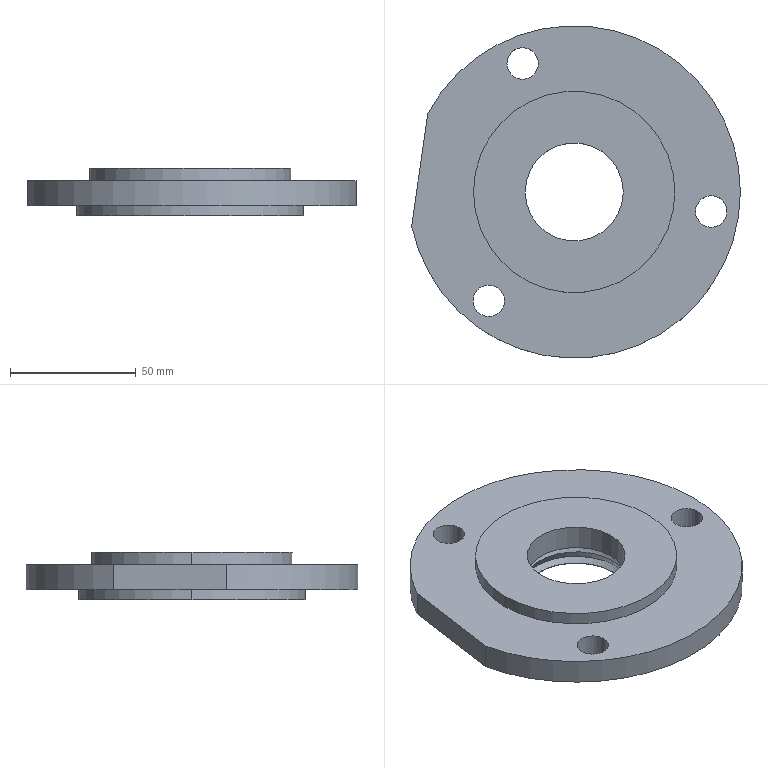Part | SolidWorks | features HoleWzd 2, Revolution 2, BaseBody 1, Extrusion 1 | 2 solids | 52 faces | box 130.573 x 132 x 19 mm | volume 150304 mm3 | cylinder 22 | torus 12 | plane 10 | cone 8 | commonest cylinder face diameters 12.5 x6 62 x4 39 x2 44.8 x2 58 x2 80 x2
STEP:
#1=CARTESIAN_POINT('',(607.231,22.744,-149.693));
#2=VERTEX_POINT('',#1);
#3=CARTESIAN_POINT('',(545.231,22.744,-149.693));
#4=VERTEX_POINT('',#3);
#5=CARTESIAN_POINT('',(576.231,22.744,-149.693));
#6=DIRECTION('',(0.,0.,-1.));
#7=DIRECTION('',(-1.,0.,0.));
#8=AXIS2_PLACEMENT_3D('',#5,#6,#7);
#9=CIRCLE('',#8,31.);
#10=EDGE_CURVE('',#2,#4,#9,.T.);
#11=ORIENTED_EDGE('',*,*,#10,.F.);
#12=CARTESIAN_POINT('',(607.231,22.744,-158.693));
#13=VERTEX_POINT('',#12);
#14=CARTESIAN_POINT('',(607.231,22.744,-158.693));
#15=DIRECTION('',(0.,0.,-1.));
#16=VECTOR('',#15,1000.);
#17=LINE('',#14,#16);
#18=EDGE_CURVE('',#2,#13,#17,.T.);
#19=ORIENTED_EDGE('',*,*,#18,.T.);
#20=CARTESIAN_POINT('',(545.231,22.744,-158.693));
#21=VERTEX_POINT('',#20);
#22=CARTESIAN_POINT('',(576.231,22.744,-158.693));
#23=DIRECTION('',(0.,0.,-1.));
#24=DIRECTION('',(-1.,0.,0.));
#25=AXIS2_PLACEMENT_3D('',#22,#23,#24);
#26=CIRCLE('',#25,31.);
#27=EDGE_CURVE('',#13,#21,#26,.T.);
#28=ORIENTED_EDGE('',*,*,#27,.T.);
#29=CARTESIAN_POINT('',(545.231,22.744,-158.693));
#30=DIRECTION('',(0.,0.,-1.));
#31=VECTOR('',#30,1000.);
#32=LINE('',#29,#31);
#33=EDGE_CURVE('',#4,#21,#32,.T.);
#34=ORIENTED_EDGE('',*,*,#33,.F.);
#35=EDGE_LOOP('',(#11,#19,#28,#34));
#36=FACE_OUTER_BOUND('',#35,.T.);
#37=CARTESIAN_POINT('',(576.231,22.744,-158.693));
#38=DIRECTION('',(0.,0.,-1.));
#39=DIRECTION('',(-1.,0.,0.));
#40=AXIS2_PLACEMENT_3D('',#37,#38,#39);
#41=CYLINDRICAL_SURFACE('',#40,31.);
#42=ADVANCED_FACE('',(#36),#41,.F.);
#43=CARTESIAN_POINT('',(595.731,22.744,-139.693));
#44=VERTEX_POINT('',#43);
#45=CARTESIAN_POINT('',(556.731,22.744,-139.693));
#46=VERTEX_POINT('',#45);
#47=CARTESIAN_POINT('',(576.231,22.744,-139.693));
#48=DIRECTION('',(0.,0.,-1.));
#49=DIRECTION('',(-1.,0.,0.));
#50=AXIS2_PLACEMENT_3D('',#47,#48,#49);
#51=CIRCLE('',#50,19.5);
#52=EDGE_CURVE('',#44,#46,#51,.T.);
#53=ORIENTED_EDGE('',*,*,#52,.F.);
#54=CARTESIAN_POINT('',(595.731,22.744,-149.693));
#55=VERTEX_POINT('',#54);
#56=CARTESIAN_POINT('',(595.731,22.744,-158.693));
#57=DIRECTION('',(0.,0.,-1.));
#58=VECTOR('',#57,1000.);
#59=LINE('',#56,#58);
#60=EDGE_CURVE('',#44,#55,#59,.T.);
#61=ORIENTED_EDGE('',*,*,#60,.T.);
#62=CARTESIAN_POINT('',(556.731,22.744,-149.693));
#63=VERTEX_POINT('',#62);
#64=CARTESIAN_POINT('',(576.231,22.744,-149.693));
#65=DIRECTION('',(0.,0.,-1.));
#66=DIRECTION('',(-1.,0.,0.));
#67=AXIS2_PLACEMENT_3D('',#64,#65,#66);
#68=CIRCLE('',#67,19.5);
#69=EDGE_CURVE('',#55,#63,#68,.T.);
#70=ORIENTED_EDGE('',*,*,#69,.T.);
#71=CARTESIAN_POINT('',(556.731,22.744,-158.693));
#72=DIRECTION('',(0.,0.,-1.));
#73=VECTOR('',#72,1000.);
#74=LINE('',#71,#73);
#75=EDGE_CURVE('',#46,#63,#74,.T.);
#76=ORIENTED_EDGE('',*,*,#75,.F.);
#77=EDGE_LOOP('',(#53,#61,#70,#76));
#78=FACE_OUTER_BOUND('',#77,.T.);
#79=CARTESIAN_POINT('',(576.231,22.744,-158.693));
#80=DIRECTION('',(0.,0.,-1.));
#81=DIRECTION('',(-1.,0.,0.));
#82=AXIS2_PLACEMENT_3D('',#79,#80,#81);
#83=CYLINDRICAL_SURFACE('',#82,19.5);
#84=ADVANCED_FACE('',(#78),#83,.F.);
#85=CARTESIAN_POINT('',(624.43,14.98,-144.693));
#86=VERTEX_POINT('',#85);
#87=CARTESIAN_POINT('',(636.93,14.98,-144.693));
#88=VERTEX_POINT('',#87);
#89=CARTESIAN_POINT('',(630.68,14.98,-144.693));
#90=DIRECTION('',(0.,0.,1.));
#91=DIRECTION('',(1.,0.,0.));
#92=AXIS2_PLACEMENT_3D('',#89,#90,#91);
#93=CIRCLE('',#92,6.25);
#94=EDGE_CURVE('',#86,#88,#93,.T.);
#95=ORIENTED_EDGE('',*,*,#94,.T.);
#96=CARTESIAN_POINT('',(636.93,14.98,-154.693));
#97=VERTEX_POINT('',#96);
#98=CARTESIAN_POINT('',(636.93,14.98,-154.693));
#99=DIRECTION('',(0.,0.,-1.));
#100=VECTOR('',#99,1000.);
#101=LINE('',#98,#100);
#102=EDGE_CURVE('',#88,#97,#101,.T.);
#103=ORIENTED_EDGE('',*,*,#102,.T.);
#104=CARTESIAN_POINT('',(624.43,14.98,-154.693));
#105=VERTEX_POINT('',#104);
#106=CARTESIAN_POINT('',(630.68,14.98,-154.693));
#107=DIRECTION('',(0.,0.,-1.));
#108=DIRECTION('',(-1.,0.,0.));
#109=AXIS2_PLACEMENT_3D('',#106,#107,#108);
#110=CIRCLE('',#109,6.25);
#111=EDGE_CURVE('',#97,#105,#110,.T.);
#112=ORIENTED_EDGE('',*,*,#111,.T.);
#113=CARTESIAN_POINT('',(624.43,14.98,-154.693));
#114=DIRECTION('',(0.,0.,-1.));
#115=VECTOR('',#114,1000.);
#116=LINE('',#113,#115);
#117=EDGE_CURVE('',#86,#105,#116,.T.);
#118=ORIENTED_EDGE('',*,*,#117,.F.);
#119=EDGE_LOOP('',(#95,#103,#112,#118));
#120=FACE_OUTER_BOUND('',#119,.T.);
#121=CARTESIAN_POINT('',(630.68,14.98,-154.693));
#122=DIRECTION('',(0.,0.,-1.));
#123=DIRECTION('',(-1.,0.,0.));
#124=AXIS2_PLACEMENT_3D('',#121,#122,#123);
#125=CYLINDRICAL_SURFACE('',#124,6.25);
#126=ADVANCED_FACE('',(#120),#125,.F.);
#127=CARTESIAN_POINT('',(536.032,-20.529,-144.693));
#128=VERTEX_POINT('',#127);
#129=CARTESIAN_POINT('',(548.532,-20.529,-144.693));
#130=VERTEX_POINT('',#129);
#131=CARTESIAN_POINT('',(542.282,-20.529,-144.693));
#132=DIRECTION('',(0.,0.,1.));
#133=DIRECTION('',(1.,0.,0.));
#134=AXIS2_PLACEMENT_3D('',#131,#132,#133);
#135=CIRCLE('',#134,6.25);
#136=EDGE_CURVE('',#128,#130,#135,.T.);
#137=ORIENTED_EDGE('',*,*,#136,.T.);
#138=CARTESIAN_POINT('',(548.532,-20.529,-154.693));
#139=VERTEX_POINT('',#138);
#140=CARTESIAN_POINT('',(548.532,-20.529,-154.693));
#141=DIRECTION('',(0.,0.,-1.));
#142=VECTOR('',#141,1000.);
#143=LINE('',#140,#142);
#144=EDGE_CURVE('',#130,#139,#143,.T.);
#145=ORIENTED_EDGE('',*,*,#144,.T.);
#146=CARTESIAN_POINT('',(536.032,-20.529,-154.693));
#147=VERTEX_POINT('',#146);
#148=CARTESIAN_POINT('',(542.282,-20.529,-154.693));
#149=DIRECTION('',(0.,0.,-1.));
#150=DIRECTION('',(-1.,0.,0.));
#151=AXIS2_PLACEMENT_3D('',#148,#149,#150);
#152=CIRCLE('',#151,6.25);
#153=EDGE_CURVE('',#139,#147,#152,.T.);
#154=ORIENTED_EDGE('',*,*,#153,.T.);
#155=CARTESIAN_POINT('',(536.032,-20.529,-154.693));
#156=DIRECTION('',(0.,0.,-1.));
#157=VECTOR('',#156,1000.);
#158=LINE('',#155,#157);
#159=EDGE_CURVE('',#128,#147,#158,.T.);
#160=ORIENTED_EDGE('',*,*,#159,.F.);
#161=EDGE_LOOP('',(#137,#145,#154,#160));
#162=FACE_OUTER_BOUND('',#161,.T.);
#163=CARTESIAN_POINT('',(542.282,-20.529,-154.693));
#164=DIRECTION('',(0.,0.,-1.));
#165=DIRECTION('',(-1.,0.,0.));
#166=AXIS2_PLACEMENT_3D('',#163,#164,#165);
#167=CYLINDRICAL_SURFACE('',#166,6.25);
#168=ADVANCED_FACE('',(#162),#167,.F.);
#169=CARTESIAN_POINT('',(549.479,73.78,-144.693));
#170=VERTEX_POINT('',#169);
#171=CARTESIAN_POINT('',(561.979,73.78,-144.693));
#172=VERTEX_POINT('',#171);
#173=CARTESIAN_POINT('',(555.729,73.78,-144.693));
#174=DIRECTION('',(0.,0.,1.));
#175=DIRECTION('',(1.,0.,0.));
#176=AXIS2_PLACEMENT_3D('',#173,#174,#175);
#177=CIRCLE('',#176,6.25);
#178=EDGE_CURVE('',#170,#172,#177,.T.);
#179=ORIENTED_EDGE('',*,*,#178,.T.);
#180=CARTESIAN_POINT('',(561.979,73.78,-154.693));
#181=VERTEX_POINT('',#180);
#182=CARTESIAN_POINT('',(561.979,73.78,-154.693));
#183=DIRECTION('',(0.,0.,-1.));
#184=VECTOR('',#183,1000.);
#185=LINE('',#182,#184);
#186=EDGE_CURVE('',#172,#181,#185,.T.);
#187=ORIENTED_EDGE('',*,*,#186,.T.);
#188=CARTESIAN_POINT('',(549.479,73.78,-154.693));
#189=VERTEX_POINT('',#188);
#190=CARTESIAN_POINT('',(555.729,73.78,-154.693));
#191=DIRECTION('',(0.,0.,-1.));
#192=DIRECTION('',(-1.,0.,0.));
#193=AXIS2_PLACEMENT_3D('',#190,#191,#192);
#194=CIRCLE('',#193,6.25);
#195=EDGE_CURVE('',#181,#189,#194,.T.);
#196=ORIENTED_EDGE('',*,*,#195,.T.);
#197=CARTESIAN_POINT('',(549.479,73.78,-154.693));
#198=DIRECTION('',(0.,0.,-1.));
#199=VECTOR('',#198,1000.);
#200=LINE('',#197,#199);
#201=EDGE_CURVE('',#170,#189,#200,.T.);
#202=ORIENTED_EDGE('',*,*,#201,.F.);
#203=EDGE_LOOP('',(#179,#187,#196,#202));
#204=FACE_OUTER_BOUND('',#203,.T.);
#205=CARTESIAN_POINT('',(555.729,73.78,-154.693));
#206=DIRECTION('',(0.,0.,-1.));
#207=DIRECTION('',(-1.,0.,0.));
#208=AXIS2_PLACEMENT_3D('',#205,#206,#207);
#209=CYLINDRICAL_SURFACE('',#208,6.25);
#210=ADVANCED_FACE('',(#204),#209,.F.);
#211=CARTESIAN_POINT('',(621.231,22.744,-158.693));
#212=VERTEX_POINT('',#211);
#213=CARTESIAN_POINT('',(531.231,22.744,-158.693));
#214=VERTEX_POINT('',#213);
#215=CARTESIAN_POINT('',(576.231,22.744,-158.693));
#216=DIRECTION('',(0.,0.,1.));
#217=DIRECTION('',(1.,0.,0.));
#218=AXIS2_PLACEMENT_3D('',#215,#216,#217);
#219=CIRCLE('',#218,45.);
#220=EDGE_CURVE('',#212,#214,#219,.T.);
#221=ORIENTED_EDGE('',*,*,#220,.T.);
#222=CARTESIAN_POINT('',(531.231,22.744,-154.693));
#223=VERTEX_POINT('',#222);
#224=CARTESIAN_POINT('',(531.231,22.744,-158.693));
#225=DIRECTION('',(0.,0.,1.));
#226=VECTOR('',#225,1000.);
#227=LINE('',#224,#226);
#228=EDGE_CURVE('',#214,#223,#227,.T.);
#229=ORIENTED_EDGE('',*,*,#228,.T.);
#230=CARTESIAN_POINT('',(621.231,22.744,-154.693));
#231=VERTEX_POINT('',#230);
#232=CARTESIAN_POINT('',(576.231,22.744,-154.693));
#233=DIRECTION('',(0.,0.,1.));
#234=DIRECTION('',(1.,0.,0.));
#235=AXIS2_PLACEMENT_3D('',#232,#233,#234);
#236=CIRCLE('',#235,45.);
#237=EDGE_CURVE('',#231,#223,#236,.T.);
#238=ORIENTED_EDGE('',*,*,#237,.F.);
#239=CARTESIAN_POINT('',(621.231,22.744,-158.693));
#240=DIRECTION('',(0.,0.,1.));
#241=VECTOR('',#240,1000.);
#242=LINE('',#239,#241);
#243=EDGE_CURVE('',#212,#231,#242,.T.);
#244=ORIENTED_EDGE('',*,*,#243,.F.);
#245=EDGE_LOOP('',(#221,#229,#238,#244));
#246=FACE_OUTER_BOUND('',#245,.T.);
#247=CARTESIAN_POINT('',(576.231,22.744,-158.693));
#248=DIRECTION('',(0.,0.,1.));
#249=DIRECTION('',(1.,0.,0.));
#250=AXIS2_PLACEMENT_3D('',#247,#248,#249);
#251=CYLINDRICAL_SURFACE('',#250,45.);
#252=ADVANCED_FACE('',(#246),#251,.T.);
#253=CARTESIAN_POINT('',(536.231,22.744,-139.693));
#254=VERTEX_POINT('',#253);
#255=CARTESIAN_POINT('',(616.231,22.744,-139.693));
#256=VERTEX_POINT('',#255);
#257=CARTESIAN_POINT('',(576.231,22.744,-139.693));
#258=DIRECTION('',(0.,0.,-1.));
#259=DIRECTION('',(-1.,0.,0.));
#260=AXIS2_PLACEMENT_3D('',#257,#258,#259);
#261=CIRCLE('',#260,40.);
#262=EDGE_CURVE('',#254,#256,#261,.T.);
#263=ORIENTED_EDGE('',*,*,#262,.T.);
#264=CARTESIAN_POINT('',(616.231,22.744,-144.693));
#265=VERTEX_POINT('',#264);
#266=CARTESIAN_POINT('',(616.231,22.744,-139.693));
#267=DIRECTION('',(0.,0.,-1.));
#268=VECTOR('',#267,1000.);
#269=LINE('',#266,#268);
#270=EDGE_CURVE('',#256,#265,#269,.T.);
#271=ORIENTED_EDGE('',*,*,#270,.T.);
#272=CARTESIAN_POINT('',(536.231,22.744,-144.693));
#273=VERTEX_POINT('',#272);
#274=CARTESIAN_POINT('',(576.231,22.744,-144.693));
#275=DIRECTION('',(0.,0.,-1.));
#276=DIRECTION('',(-1.,0.,0.));
#277=AXIS2_PLACEMENT_3D('',#274,#275,#276);
#278=CIRCLE('',#277,40.);
#279=EDGE_CURVE('',#273,#265,#278,.T.);
#280=ORIENTED_EDGE('',*,*,#279,.F.);
#281=CARTESIAN_POINT('',(536.231,22.744,-139.693));
#282=DIRECTION('',(0.,0.,-1.));
#283=VECTOR('',#282,1000.);
#284=LINE('',#281,#283);
#285=EDGE_CURVE('',#254,#273,#284,.T.);
#286=ORIENTED_EDGE('',*,*,#285,.F.);
#287=EDGE_LOOP('',(#263,#271,#280,#286));
#288=FACE_OUTER_BOUND('',#287,.T.);
#289=CARTESIAN_POINT('',(576.231,22.744,-139.693));
#290=DIRECTION('',(0.,0.,-1.));
#291=DIRECTION('',(-1.,0.,0.));
#292=AXIS2_PLACEMENT_3D('',#289,#290,#291);
#293=CYLINDRICAL_SURFACE('',#292,40.);
#294=ADVANCED_FACE('',(#288),#293,.T.);
#295=CARTESIAN_POINT('',(511.657,9.095,-154.693));
#296=VERTEX_POINT('',#295);
#297=CARTESIAN_POINT('',(642.231,22.744,-154.693));
#298=VERTEX_POINT('',#297);
#299=CARTESIAN_POINT('',(576.231,22.744,-154.693));
#300=DIRECTION('',(0.,0.,1.));
#301=DIRECTION('',(1.,0.,0.));
#302=AXIS2_PLACEMENT_3D('',#299,#300,#301);
#303=CIRCLE('',#302,66.);
#304=EDGE_CURVE('',#296,#298,#303,.T.);
#305=ORIENTED_EDGE('',*,*,#304,.T.);
#306=CARTESIAN_POINT('',(642.231,22.744,-144.693));
#307=VERTEX_POINT('',#306);
#308=CARTESIAN_POINT('',(642.231,22.744,-154.693));
#309=DIRECTION('',(0.,0.,1.));
#310=VECTOR('',#309,1000.);
#311=LINE('',#308,#310);
#312=EDGE_CURVE('',#298,#307,#311,.T.);
#313=ORIENTED_EDGE('',*,*,#312,.T.);
#314=CARTESIAN_POINT('',(511.657,9.095,-144.693));
#315=VERTEX_POINT('',#314);
#316=CARTESIAN_POINT('',(576.231,22.744,-144.693));
#317=DIRECTION('',(0.,0.,1.));
#318=DIRECTION('',(1.,0.,0.));
#319=AXIS2_PLACEMENT_3D('',#316,#317,#318);
#320=CIRCLE('',#319,66.);
#321=EDGE_CURVE('',#315,#307,#320,.T.);
#322=ORIENTED_EDGE('',*,*,#321,.F.);
#323=CARTESIAN_POINT('',(511.657,9.095,-154.693));
#324=DIRECTION('',(0.,0.,1.));
#325=VECTOR('',#324,1000.);
#326=LINE('',#323,#325);
#327=EDGE_CURVE('',#296,#315,#326,.T.);
#328=ORIENTED_EDGE('',*,*,#327,.F.);
#329=EDGE_LOOP('',(#305,#313,#322,#328));
#330=FACE_OUTER_BOUND('',#329,.T.);
#331=CARTESIAN_POINT('',(576.231,22.744,-154.693));
#332=DIRECTION('',(0.,0.,1.));
#333=DIRECTION('',(1.,0.,0.));
#334=AXIS2_PLACEMENT_3D('',#331,#332,#333);
#335=CYLINDRICAL_SURFACE('',#334,66.);
#336=ADVANCED_FACE('',(#330),#335,.T.);
#337=ORIENTED_EDGE('',*,*,#312,.F.);
#338=CARTESIAN_POINT('',(518.045,53.897,-154.693));
#339=VERTEX_POINT('',#338);
#340=CARTESIAN_POINT('',(576.231,22.744,-154.693));
#341=DIRECTION('',(0.,0.,1.));
#342=DIRECTION('',(1.,0.,0.));
#343=AXIS2_PLACEMENT_3D('',#340,#341,#342);
#344=CIRCLE('',#343,66.);
#345=EDGE_CURVE('',#298,#339,#344,.T.);
#346=ORIENTED_EDGE('',*,*,#345,.T.);
#347=CARTESIAN_POINT('',(518.045,53.897,-144.693));
#348=VERTEX_POINT('',#347);
#349=CARTESIAN_POINT('',(518.045,53.897,-154.693));
#350=DIRECTION('',(0.,0.,1.));
#351=VECTOR('',#350,1000.);
#352=LINE('',#349,#351);
#353=EDGE_CURVE('',#339,#348,#352,.T.);
#354=ORIENTED_EDGE('',*,*,#353,.T.);
#355=CARTESIAN_POINT('',(576.231,22.744,-144.693));
#356=DIRECTION('',(0.,0.,1.));
#357=DIRECTION('',(1.,0.,0.));
#358=AXIS2_PLACEMENT_3D('',#355,#356,#357);
#359=CIRCLE('',#358,66.);
#360=EDGE_CURVE('',#307,#348,#359,.T.);
#361=ORIENTED_EDGE('',*,*,#360,.F.);
#362=EDGE_LOOP('',(#337,#346,#354,#361));
#363=FACE_OUTER_BOUND('',#362,.T.);
#364=CARTESIAN_POINT('',(576.231,22.744,-154.693));
#365=DIRECTION('',(0.,0.,1.));
#366=DIRECTION('',(1.,0.,0.));
#367=AXIS2_PLACEMENT_3D('',#364,#365,#366);
#368=CYLINDRICAL_SURFACE('',#367,66.);
#369=ADVANCED_FACE('',(#363),#368,.T.);
#370=CARTESIAN_POINT('',(518.045,53.897,-144.693));
#371=DIRECTION('',(-0.1412,-0.99,0.));
#372=VECTOR('',#371,1000.);
#373=LINE('',#370,#372);
#374=EDGE_CURVE('',#348,#315,#373,.T.);
#375=ORIENTED_EDGE('',*,*,#374,.F.);
#376=ORIENTED_EDGE('',*,*,#353,.F.);
#377=CARTESIAN_POINT('',(518.045,53.897,-154.693));
#378=DIRECTION('',(-0.1412,-0.99,0.));
#379=VECTOR('',#378,1000.);
#380=LINE('',#377,#379);
#381=EDGE_CURVE('',#339,#296,#380,.T.);
#382=ORIENTED_EDGE('',*,*,#381,.T.);
#383=ORIENTED_EDGE('',*,*,#327,.T.);
#384=EDGE_LOOP('',(#375,#376,#382,#383));
#385=FACE_OUTER_BOUND('',#384,.T.);
#386=CARTESIAN_POINT('',(518.045,53.897,-154.693));
#387=DIRECTION('',(-0.99,0.1412,0.));
#388=DIRECTION('',(-0.1412,-0.99,0.));
#389=AXIS2_PLACEMENT_3D('',#386,#387,#388);
#390=PLANE('',#389);
#391=ADVANCED_FACE('',(#385),#390,.T.);
#392=CARTESIAN_POINT('',(630.68,14.98,-154.693));
#393=DIRECTION('',(0.,0.,-1.));
#394=DIRECTION('',(-1.,0.,0.));
#395=AXIS2_PLACEMENT_3D('',#392,#393,#394);
#396=CIRCLE('',#395,6.25);
#397=EDGE_CURVE('',#105,#97,#396,.T.);
#398=ORIENTED_EDGE('',*,*,#397,.F.);
#399=ORIENTED_EDGE('',*,*,#111,.F.);
#400=EDGE_LOOP('',(#398,#399));
#401=FACE_BOUND('',#400,.T.);
#402=CARTESIAN_POINT('',(542.282,-20.529,-154.693));
#403=DIRECTION('',(0.,0.,-1.));
#404=DIRECTION('',(-1.,0.,0.));
#405=AXIS2_PLACEMENT_3D('',#402,#403,#404);
#406=CIRCLE('',#405,6.25);
#407=EDGE_CURVE('',#147,#139,#406,.T.);
#408=ORIENTED_EDGE('',*,*,#407,.F.);
#409=ORIENTED_EDGE('',*,*,#153,.F.);
#410=EDGE_LOOP('',(#408,#409));
#411=FACE_BOUND('',#410,.T.);
#412=CARTESIAN_POINT('',(555.729,73.78,-154.693));
#413=DIRECTION('',(0.,0.,-1.));
#414=DIRECTION('',(-1.,0.,0.));
#415=AXIS2_PLACEMENT_3D('',#412,#413,#414);
#416=CIRCLE('',#415,6.25);
#417=EDGE_CURVE('',#189,#181,#416,.T.);
#418=ORIENTED_EDGE('',*,*,#417,.F.);
#419=ORIENTED_EDGE('',*,*,#195,.F.);
#420=EDGE_LOOP('',(#418,#419));
#421=FACE_BOUND('',#420,.T.);
#422=ORIENTED_EDGE('',*,*,#237,.T.);
#423=CARTESIAN_POINT('',(576.231,22.744,-154.693));
#424=DIRECTION('',(0.,0.,1.));
#425=DIRECTION('',(1.,0.,0.));
#426=AXIS2_PLACEMENT_3D('',#423,#424,#425);
#427=CIRCLE('',#426,45.);
#428=EDGE_CURVE('',#223,#231,#427,.T.);
#429=ORIENTED_EDGE('',*,*,#428,.T.);
#430=EDGE_LOOP('',(#422,#429));
#431=FACE_BOUND('',#430,.T.);
#432=ORIENTED_EDGE('',*,*,#304,.F.);
#433=ORIENTED_EDGE('',*,*,#381,.F.);
#434=ORIENTED_EDGE('',*,*,#345,.F.);
#435=EDGE_LOOP('',(#432,#433,#434));
#436=FACE_OUTER_BOUND('',#435,.T.);
#437=CARTESIAN_POINT('',(576.231,22.744,-154.693));
#438=DIRECTION('',(0.,0.,1.));
#439=DIRECTION('',(1.,0.,0.));
#440=AXIS2_PLACEMENT_3D('',#437,#438,#439);
#441=PLANE('',#440);
#442=ADVANCED_FACE('',(#401,#411,#421,#431,#436),#441,.F.);
#443=ORIENTED_EDGE('',*,*,#94,.F.);
#444=CARTESIAN_POINT('',(630.68,14.98,-144.693));
#445=DIRECTION('',(0.,0.,1.));
#446=DIRECTION('',(1.,0.,0.));
#447=AXIS2_PLACEMENT_3D('',#444,#445,#446);
#448=CIRCLE('',#447,6.25);
#449=EDGE_CURVE('',#88,#86,#448,.T.);
#450=ORIENTED_EDGE('',*,*,#449,.F.);
#451=EDGE_LOOP('',(#443,#450));
#452=FACE_BOUND('',#451,.T.);
#453=ORIENTED_EDGE('',*,*,#136,.F.);
#454=CARTESIAN_POINT('',(542.282,-20.529,-144.693));
#455=DIRECTION('',(0.,0.,1.));
#456=DIRECTION('',(1.,0.,0.));
#457=AXIS2_PLACEMENT_3D('',#454,#455,#456);
#458=CIRCLE('',#457,6.25);
#459=EDGE_CURVE('',#130,#128,#458,.T.);
#460=ORIENTED_EDGE('',*,*,#459,.F.);
#461=EDGE_LOOP('',(#453,#460));
#462=FACE_BOUND('',#461,.T.);
#463=ORIENTED_EDGE('',*,*,#178,.F.);
#464=CARTESIAN_POINT('',(555.729,73.78,-144.693));
#465=DIRECTION('',(0.,0.,1.));
#466=DIRECTION('',(1.,0.,0.));
#467=AXIS2_PLACEMENT_3D('',#464,#465,#466);
#468=CIRCLE('',#467,6.25);
#469=EDGE_CURVE('',#172,#170,#468,.T.);
#470=ORIENTED_EDGE('',*,*,#469,.F.);
#471=EDGE_LOOP('',(#463,#470));
#472=FACE_BOUND('',#471,.T.);
#473=ORIENTED_EDGE('',*,*,#279,.T.);
#474=CARTESIAN_POINT('',(576.231,22.744,-144.693));
#475=DIRECTION('',(0.,0.,-1.));
#476=DIRECTION('',(-1.,0.,0.));
#477=AXIS2_PLACEMENT_3D('',#474,#475,#476);
#478=CIRCLE('',#477,40.);
#479=EDGE_CURVE('',#265,#273,#478,.T.);
#480=ORIENTED_EDGE('',*,*,#479,.T.);
#481=EDGE_LOOP('',(#473,#480));
#482=FACE_BOUND('',#481,.T.);
#483=ORIENTED_EDGE('',*,*,#321,.T.);
#484=ORIENTED_EDGE('',*,*,#360,.T.);
#485=ORIENTED_EDGE('',*,*,#374,.T.);
#486=EDGE_LOOP('',(#483,#484,#485));
#487=FACE_OUTER_BOUND('',#486,.T.);
#488=CARTESIAN_POINT('',(576.231,22.744,-144.693));
#489=DIRECTION('',(0.,0.,1.));
#490=DIRECTION('',(1.,0.,0.));
#491=AXIS2_PLACEMENT_3D('',#488,#489,#490);
#492=PLANE('',#491);
#493=ADVANCED_FACE('',(#452,#462,#472,#482,#487),#492,.T.);
#494=ORIENTED_EDGE('',*,*,#270,.F.);
#495=CARTESIAN_POINT('',(576.231,22.744,-139.693));
#496=DIRECTION('',(0.,0.,-1.));
#497=DIRECTION('',(-1.,0.,0.));
#498=AXIS2_PLACEMENT_3D('',#495,#496,#497);
#499=CIRCLE('',#498,40.);
#500=EDGE_CURVE('',#256,#254,#499,.T.);
#501=ORIENTED_EDGE('',*,*,#500,.T.);
#502=ORIENTED_EDGE('',*,*,#285,.T.);
#503=ORIENTED_EDGE('',*,*,#479,.F.);
#504=EDGE_LOOP('',(#494,#501,#502,#503));
#505=FACE_OUTER_BOUND('',#504,.T.);
#506=CARTESIAN_POINT('',(576.231,22.744,-139.693));
#507=DIRECTION('',(0.,0.,-1.));
#508=DIRECTION('',(-1.,0.,0.));
#509=AXIS2_PLACEMENT_3D('',#506,#507,#508);
#510=CYLINDRICAL_SURFACE('',#509,40.);
#511=ADVANCED_FACE('',(#505),#510,.T.);
#512=CARTESIAN_POINT('',(576.231,22.744,-139.693));
#513=DIRECTION('',(0.,0.,-1.));
#514=DIRECTION('',(-1.,0.,0.));
#515=AXIS2_PLACEMENT_3D('',#512,#513,#514);
#516=CIRCLE('',#515,19.5);
#517=EDGE_CURVE('',#46,#44,#516,.T.);
#518=ORIENTED_EDGE('',*,*,#517,.T.);
#519=ORIENTED_EDGE('',*,*,#52,.T.);
#520=EDGE_LOOP('',(#518,#519));
#521=FACE_BOUND('',#520,.T.);
#522=ORIENTED_EDGE('',*,*,#262,.F.);
#523=ORIENTED_EDGE('',*,*,#500,.F.);
#524=EDGE_LOOP('',(#522,#523));
#525=FACE_OUTER_BOUND('',#524,.T.);
#526=CARTESIAN_POINT('',(616.231,22.744,-139.693));
#527=DIRECTION('',(0.,0.,1.));
#528=DIRECTION('',(1.,0.,0.));
#529=AXIS2_PLACEMENT_3D('',#526,#527,#528);
#530=PLANE('',#529);
#531=ADVANCED_FACE('',(#521,#525),#530,.T.);
#532=ORIENTED_EDGE('',*,*,#228,.F.);
#533=CARTESIAN_POINT('',(576.231,22.744,-158.693));
#534=DIRECTION('',(0.,0.,1.));
#535=DIRECTION('',(1.,0.,0.));
#536=AXIS2_PLACEMENT_3D('',#533,#534,#535);
#537=CIRCLE('',#536,45.);
#538=EDGE_CURVE('',#214,#212,#537,.T.);
#539=ORIENTED_EDGE('',*,*,#538,.T.);
#540=ORIENTED_EDGE('',*,*,#243,.T.);
#541=ORIENTED_EDGE('',*,*,#428,.F.);
#542=EDGE_LOOP('',(#532,#539,#540,#541));
#543=FACE_OUTER_BOUND('',#542,.T.);
#544=CARTESIAN_POINT('',(576.231,22.744,-158.693));
#545=DIRECTION('',(0.,0.,1.));
#546=DIRECTION('',(1.,0.,0.));
#547=AXIS2_PLACEMENT_3D('',#544,#545,#546);
#548=CYLINDRICAL_SURFACE('',#547,45.);
#549=ADVANCED_FACE('',(#543),#548,.T.);
#550=CARTESIAN_POINT('',(576.231,22.744,-158.693));
#551=DIRECTION('',(0.,0.,-1.));
#552=DIRECTION('',(-1.,0.,0.));
#553=AXIS2_PLACEMENT_3D('',#550,#551,#552);
#554=CIRCLE('',#553,31.);
#555=EDGE_CURVE('',#21,#13,#554,.T.);
#556=ORIENTED_EDGE('',*,*,#555,.F.);
#557=ORIENTED_EDGE('',*,*,#27,.F.);
#558=EDGE_LOOP('',(#556,#557));
#559=FACE_BOUND('',#558,.T.);
#560=ORIENTED_EDGE('',*,*,#220,.F.);
#561=ORIENTED_EDGE('',*,*,#538,.F.);
#562=EDGE_LOOP('',(#560,#561));
#563=FACE_OUTER_BOUND('',#562,.T.);
#564=CARTESIAN_POINT('',(621.231,22.744,-158.693));
#565=DIRECTION('',(0.,0.,-1.));
#566=DIRECTION('',(-1.,0.,0.));
#567=AXIS2_PLACEMENT_3D('',#564,#565,#566);
#568=PLANE('',#567);
#569=ADVANCED_FACE('',(#559,#563),#568,.T.);
#570=ORIENTED_EDGE('',*,*,#186,.F.);
#571=ORIENTED_EDGE('',*,*,#469,.T.);
#572=ORIENTED_EDGE('',*,*,#201,.T.);
#573=ORIENTED_EDGE('',*,*,#417,.T.);
#574=EDGE_LOOP('',(#570,#571,#572,#573));
#575=FACE_OUTER_BOUND('',#574,.T.);
#576=CARTESIAN_POINT('',(555.729,73.78,-154.693));
#577=DIRECTION('',(0.,0.,-1.));
#578=DIRECTION('',(-1.,0.,0.));
#579=AXIS2_PLACEMENT_3D('',#576,#577,#578);
#580=CYLINDRICAL_SURFACE('',#579,6.25);
#581=ADVANCED_FACE('',(#575),#580,.F.);
#582=ORIENTED_EDGE('',*,*,#144,.F.);
#583=ORIENTED_EDGE('',*,*,#459,.T.);
#584=ORIENTED_EDGE('',*,*,#159,.T.);
#585=ORIENTED_EDGE('',*,*,#407,.T.);
#586=EDGE_LOOP('',(#582,#583,#584,#585));
#587=FACE_OUTER_BOUND('',#586,.T.);
#588=CARTESIAN_POINT('',(542.282,-20.529,-154.693));
#589=DIRECTION('',(0.,0.,-1.));
#590=DIRECTION('',(-1.,0.,0.));
#591=AXIS2_PLACEMENT_3D('',#588,#589,#590);
#592=CYLINDRICAL_SURFACE('',#591,6.25);
#593=ADVANCED_FACE('',(#587),#592,.F.);
#594=ORIENTED_EDGE('',*,*,#102,.F.);
#595=ORIENTED_EDGE('',*,*,#449,.T.);
#596=ORIENTED_EDGE('',*,*,#117,.T.);
#597=ORIENTED_EDGE('',*,*,#397,.T.);
#598=EDGE_LOOP('',(#594,#595,#596,#597));
#599=FACE_OUTER_BOUND('',#598,.T.);
#600=CARTESIAN_POINT('',(630.68,14.98,-154.693));
#601=DIRECTION('',(0.,0.,-1.));
#602=DIRECTION('',(-1.,0.,0.));
#603=AXIS2_PLACEMENT_3D('',#600,#601,#602);
#604=CYLINDRICAL_SURFACE('',#603,6.25);
#605=ADVANCED_FACE('',(#599),#604,.F.);
#606=ORIENTED_EDGE('',*,*,#60,.F.);
#607=ORIENTED_EDGE('',*,*,#517,.F.);
#608=ORIENTED_EDGE('',*,*,#75,.T.);
#609=CARTESIAN_POINT('',(576.231,22.744,-149.693));
#610=DIRECTION('',(0.,0.,-1.));
#611=DIRECTION('',(-1.,0.,0.));
#612=AXIS2_PLACEMENT_3D('',#609,#610,#611);
#613=CIRCLE('',#612,19.5);
#614=EDGE_CURVE('',#63,#55,#613,.T.);
#615=ORIENTED_EDGE('',*,*,#614,.T.);
#616=EDGE_LOOP('',(#606,#607,#608,#615));
#617=FACE_OUTER_BOUND('',#616,.T.);
#618=CARTESIAN_POINT('',(576.231,22.744,-158.693));
#619=DIRECTION('',(0.,0.,-1.));
#620=DIRECTION('',(-1.,0.,0.));
#621=AXIS2_PLACEMENT_3D('',#618,#619,#620);
#622=CYLINDRICAL_SURFACE('',#621,19.5);
#623=ADVANCED_FACE('',(#617),#622,.F.);
#624=ORIENTED_EDGE('',*,*,#614,.F.);
#625=ORIENTED_EDGE('',*,*,#69,.F.);
#626=EDGE_LOOP('',(#624,#625));
#627=FACE_BOUND('',#626,.T.);
#628=CARTESIAN_POINT('',(576.231,22.744,-149.693));
#629=DIRECTION('',(0.,0.,-1.));
#630=DIRECTION('',(-1.,0.,0.));
#631=AXIS2_PLACEMENT_3D('',#628,#629,#630);
#632=CIRCLE('',#631,31.);
#633=EDGE_CURVE('',#4,#2,#632,.T.);
#634=ORIENTED_EDGE('',*,*,#633,.T.);
#635=ORIENTED_EDGE('',*,*,#10,.T.);
#636=EDGE_LOOP('',(#634,#635));
#637=FACE_OUTER_BOUND('',#636,.T.);
#638=CARTESIAN_POINT('',(595.731,22.744,-149.693));
#639=DIRECTION('',(0.,0.,1.));
#640=DIRECTION('',(1.,0.,0.));
#641=AXIS2_PLACEMENT_3D('',#638,#639,#640);
#642=PLANE('',#641);
#643=ADVANCED_FACE('',(#627,#637),#642,.F.);
#644=ORIENTED_EDGE('',*,*,#18,.F.);
#645=ORIENTED_EDGE('',*,*,#633,.F.);
#646=ORIENTED_EDGE('',*,*,#33,.T.);
#647=ORIENTED_EDGE('',*,*,#555,.T.);
#648=EDGE_LOOP('',(#644,#645,#646,#647));
#649=FACE_OUTER_BOUND('',#648,.T.);
#650=CARTESIAN_POINT('',(576.231,22.744,-158.693));
#651=DIRECTION('',(0.,0.,-1.));
#652=DIRECTION('',(-1.,0.,0.));
#653=AXIS2_PLACEMENT_3D('',#650,#651,#652);
#654=CYLINDRICAL_SURFACE('',#653,31.);
#655=ADVANCED_FACE('',(#649),#654,.F.);
#656=CLOSED_SHELL('',(#42,#84,#126,#168,#210,#252,#294,#336,#369,#391,#442,#493,#511,#531,#549,#569,#581,#593,#605,#623,#643,#655));
#657=MANIFOLD_SOLID_BREP('',#656);
#658=CARTESIAN_POINT('',(591.139,9.412,-157.604));
#659=VERTEX_POINT('',#658);
#660=CARTESIAN_POINT('',(591.16,9.394,-157.539));
#661=VERTEX_POINT('',#660);
#662=CARTESIAN_POINT('',(591.206,9.353,-157.604));
#663=DIRECTION('',(0.6666,0.7454,0.));
#664=DIRECTION('',(-0.7454,0.6666,0.));
#665=AXIS2_PLACEMENT_3D('',#662,#663,#664);
#666=CIRCLE('',#665,0.08889);
#667=EDGE_CURVE('',#659,#661,#666,.T.);
#668=ORIENTED_EDGE('',*,*,#667,.F.);
#669=CARTESIAN_POINT('',(561.322,36.076,-157.604));
#670=VERTEX_POINT('',#669);
#671=CARTESIAN_POINT('',(576.231,22.744,-157.604));
#672=DIRECTION('',(0.,0.,-1.));
#673=DIRECTION('',(-1.,0.,0.));
#674=AXIS2_PLACEMENT_3D('',#671,#672,#673);
#675=CIRCLE('',#674,20.);
#676=EDGE_CURVE('',#659,#670,#675,.T.);
#677=ORIENTED_EDGE('',*,*,#676,.T.);
#678=CARTESIAN_POINT('',(561.301,36.094,-157.539));
#679=VERTEX_POINT('',#678);
#680=CARTESIAN_POINT('',(561.256,36.135,-157.604));
#681=DIRECTION('',(-0.6666,-0.7454,0.));
#682=DIRECTION('',(0.7454,-0.6666,0.));
#683=AXIS2_PLACEMENT_3D('',#680,#681,#682);
#684=CIRCLE('',#683,0.08889);
#685=EDGE_CURVE('',#670,#679,#684,.T.);
#686=ORIENTED_EDGE('',*,*,#685,.T.);
#687=CARTESIAN_POINT('',(576.231,22.744,-157.539));
#688=DIRECTION('',(0.,0.,-1.));
#689=DIRECTION('',(-0.7454,0.6666,0.));
#690=AXIS2_PLACEMENT_3D('',#687,#688,#689);
#691=CIRCLE('',#690,20.028);
#692=EDGE_CURVE('',#661,#679,#691,.T.);
#693=ORIENTED_EDGE('',*,*,#692,.F.);
#694=EDGE_LOOP('',(#668,#677,#686,#693));
#695=FACE_OUTER_BOUND('',#694,.T.);
#696=CARTESIAN_POINT('',(576.231,22.744,-157.604));
#697=DIRECTION('',(0.,0.,-1.));
#698=DIRECTION('',(-0.7454,0.6666,0.));
#699=AXIS2_PLACEMENT_3D('',#696,#697,#698);
#700=TOROIDAL_SURFACE('',#699,20.089,0.08889);
#701=ADVANCED_FACE('',(#695),#700,.T.);
#702=ORIENTED_EDGE('',*,*,#685,.F.);
#703=CARTESIAN_POINT('',(576.231,22.744,-157.604));
#704=DIRECTION('',(0.,0.,-1.));
#705=DIRECTION('',(-1.,0.,0.));
#706=AXIS2_PLACEMENT_3D('',#703,#704,#705);
#707=CIRCLE('',#706,20.);
#708=EDGE_CURVE('',#670,#659,#707,.T.);
#709=ORIENTED_EDGE('',*,*,#708,.T.);
#710=ORIENTED_EDGE('',*,*,#667,.T.);
#711=CARTESIAN_POINT('',(576.231,22.744,-157.539));
#712=DIRECTION('',(0.,0.,-1.));
#713=DIRECTION('',(-0.7454,0.6666,0.));
#714=AXIS2_PLACEMENT_3D('',#711,#712,#713);
#715=CIRCLE('',#714,20.028);
#716=EDGE_CURVE('',#679,#661,#715,.T.);
#717=ORIENTED_EDGE('',*,*,#716,.F.);
#718=EDGE_LOOP('',(#702,#709,#710,#717));
#719=FACE_OUTER_BOUND('',#718,.T.);
#720=CARTESIAN_POINT('',(576.231,22.744,-157.604));
#721=DIRECTION('',(0.,0.,-1.));
#722=DIRECTION('',(-0.7454,0.6666,0.));
#723=AXIS2_PLACEMENT_3D('',#720,#721,#722);
#724=TOROIDAL_SURFACE('',#723,20.089,0.08889);
#725=ADVANCED_FACE('',(#719),#724,.T.);
#726=CARTESIAN_POINT('',(591.139,9.412,-152.093));
#727=VERTEX_POINT('',#726);
#728=CARTESIAN_POINT('',(561.322,36.076,-152.093));
#729=VERTEX_POINT('',#728);
#730=CARTESIAN_POINT('',(576.231,22.744,-152.093));
#731=DIRECTION('',(0.,0.,-1.));
#732=DIRECTION('',(-0.7454,0.6666,0.));
#733=AXIS2_PLACEMENT_3D('',#730,#731,#732);
#734=CIRCLE('',#733,20.);
#735=EDGE_CURVE('',#727,#729,#734,.T.);
#736=ORIENTED_EDGE('',*,*,#735,.T.);
#737=CARTESIAN_POINT('',(560.605,36.716,-150.493));
#738=VERTEX_POINT('',#737);
#739=CARTESIAN_POINT('',(561.322,36.076,-152.093));
#740=DIRECTION('',(-0.3839,0.3433,0.8572));
#741=VECTOR('',#740,1000.);
#742=LINE('',#739,#741);
#743=EDGE_CURVE('',#729,#738,#742,.T.);
#744=ORIENTED_EDGE('',*,*,#743,.T.);
#745=CARTESIAN_POINT('',(591.856,8.771,-150.493));
#746=VERTEX_POINT('',#745);
#747=CARTESIAN_POINT('',(576.231,22.744,-150.493));
#748=DIRECTION('',(0.,0.,-1.));
#749=DIRECTION('',(-0.7454,0.6666,0.));
#750=AXIS2_PLACEMENT_3D('',#747,#748,#749);
#751=CIRCLE('',#750,20.961);
#752=EDGE_CURVE('',#746,#738,#751,.T.);
#753=ORIENTED_EDGE('',*,*,#752,.F.);
#754=CARTESIAN_POINT('',(591.139,9.412,-152.093));
#755=DIRECTION('',(0.3839,-0.3433,0.8572));
#756=VECTOR('',#755,1000.);
#757=LINE('',#754,#756);
#758=EDGE_CURVE('',#727,#746,#757,.T.);
#759=ORIENTED_EDGE('',*,*,#758,.F.);
#760=EDGE_LOOP('',(#736,#744,#753,#759));
#761=FACE_OUTER_BOUND('',#760,.T.);
#762=CARTESIAN_POINT('',(576.231,22.744,-152.093));
#763=DIRECTION('',(0.,0.,1.));
#764=DIRECTION('',(0.7454,-0.6666,0.));
#765=AXIS2_PLACEMENT_3D('',#762,#763,#764);
#766=CONICAL_SURFACE('',#765,20.,0.5411);
#767=ADVANCED_FACE('',(#761),#766,.F.);
#768=ORIENTED_EDGE('',*,*,#735,.F.);
#769=CARTESIAN_POINT('',(592.63,8.079,-155.693));
#770=VERTEX_POINT('',#769);
#771=CARTESIAN_POINT('',(592.63,8.079,-155.693));
#772=DIRECTION('',(0.362,-0.3237,-0.8742));
#773=VECTOR('',#772,1000.);
#774=LINE('',#771,#773);
#775=EDGE_CURVE('',#727,#770,#774,.T.);
#776=ORIENTED_EDGE('',*,*,#775,.T.);
#777=CARTESIAN_POINT('',(559.831,37.409,-155.693));
#778=VERTEX_POINT('',#777);
#779=CARTESIAN_POINT('',(576.231,22.744,-155.693));
#780=DIRECTION('',(0.,0.,-1.));
#781=DIRECTION('',(-0.7454,0.6666,0.));
#782=AXIS2_PLACEMENT_3D('',#779,#780,#781);
#783=CIRCLE('',#782,22.);
#784=EDGE_CURVE('',#770,#778,#783,.T.);
#785=ORIENTED_EDGE('',*,*,#784,.T.);
#786=CARTESIAN_POINT('',(559.831,37.409,-155.693));
#787=DIRECTION('',(-0.362,0.3237,-0.8742));
#788=VECTOR('',#787,1000.);
#789=LINE('',#786,#788);
#790=EDGE_CURVE('',#729,#778,#789,.T.);
#791=ORIENTED_EDGE('',*,*,#790,.F.);
#792=EDGE_LOOP('',(#768,#776,#785,#791));
#793=FACE_OUTER_BOUND('',#792,.T.);
#794=CARTESIAN_POINT('',(576.231,22.744,-155.693));
#795=DIRECTION('',(0.,0.,-1.));
#796=DIRECTION('',(-0.7454,0.6666,0.));
#797=AXIS2_PLACEMENT_3D('',#794,#795,#796);
#798=CONICAL_SURFACE('',#797,22.,0.5071);
#799=ADVANCED_FACE('',(#793),#798,.F.);
#800=ORIENTED_EDGE('',*,*,#692,.T.);
#801=CARTESIAN_POINT('',(561.301,36.094,-157.539));
#802=DIRECTION('',(-0.5441,0.4866,0.6835));
#803=VECTOR('',#802,1000.);
#804=LINE('',#801,#803);
#805=EDGE_CURVE('',#679,#778,#804,.T.);
#806=ORIENTED_EDGE('',*,*,#805,.T.);
#807=ORIENTED_EDGE('',*,*,#784,.F.);
#808=CARTESIAN_POINT('',(591.16,9.394,-157.539));
#809=DIRECTION('',(0.5441,-0.4866,0.6835));
#810=VECTOR('',#809,1000.);
#811=LINE('',#808,#810);
#812=EDGE_CURVE('',#661,#770,#811,.T.);
#813=ORIENTED_EDGE('',*,*,#812,.F.);
#814=EDGE_LOOP('',(#800,#806,#807,#813));
#815=FACE_OUTER_BOUND('',#814,.T.);
#816=CARTESIAN_POINT('',(576.231,22.744,-157.539));
#817=DIRECTION('',(0.,0.,1.));
#818=DIRECTION('',(0.7454,-0.6666,0.));
#819=AXIS2_PLACEMENT_3D('',#816,#817,#818);
#820=CONICAL_SURFACE('',#819,20.028,0.8183);
#821=ADVANCED_FACE('',(#815),#820,.F.);
#822=ORIENTED_EDGE('',*,*,#708,.F.);
#823=CARTESIAN_POINT('',(561.256,36.135,-157.693));
#824=VERTEX_POINT('',#823);
#825=CARTESIAN_POINT('',(561.256,36.135,-157.604));
#826=DIRECTION('',(-0.6666,-0.7454,0.));
#827=DIRECTION('',(0.7454,-0.6666,0.));
#828=AXIS2_PLACEMENT_3D('',#825,#826,#827);
#829=CIRCLE('',#828,0.08889);
#830=EDGE_CURVE('',#824,#670,#829,.T.);
#831=ORIENTED_EDGE('',*,*,#830,.F.);
#832=CARTESIAN_POINT('',(591.206,9.353,-157.693));
#833=VERTEX_POINT('',#832);
#834=CARTESIAN_POINT('',(576.231,22.744,-157.693));
#835=DIRECTION('',(0.,0.,-1.));
#836=DIRECTION('',(-0.7454,0.6666,0.));
#837=AXIS2_PLACEMENT_3D('',#834,#835,#836);
#838=CIRCLE('',#837,20.089);
#839=EDGE_CURVE('',#824,#833,#838,.T.);
#840=ORIENTED_EDGE('',*,*,#839,.T.);
#841=CARTESIAN_POINT('',(591.206,9.353,-157.604));
#842=DIRECTION('',(0.6666,0.7454,0.));
#843=DIRECTION('',(-0.7454,0.6666,0.));
#844=AXIS2_PLACEMENT_3D('',#841,#842,#843);
#845=CIRCLE('',#844,0.08889);
#846=EDGE_CURVE('',#833,#659,#845,.T.);
#847=ORIENTED_EDGE('',*,*,#846,.T.);
#848=EDGE_LOOP('',(#822,#831,#840,#847));
#849=FACE_OUTER_BOUND('',#848,.T.);
#850=CARTESIAN_POINT('',(576.231,22.744,-157.604));
#851=DIRECTION('',(0.,0.,-1.));
#852=DIRECTION('',(-0.7454,0.6666,0.));
#853=AXIS2_PLACEMENT_3D('',#850,#851,#852);
#854=TOROIDAL_SURFACE('',#853,20.089,0.08889);
#855=ADVANCED_FACE('',(#849),#854,.T.);
#856=CARTESIAN_POINT('',(553.122,43.408,-157.293));
#857=VERTEX_POINT('',#856);
#858=CARTESIAN_POINT('',(599.339,2.08,-157.293));
#859=VERTEX_POINT('',#858);
#860=CARTESIAN_POINT('',(576.231,22.744,-157.293));
#861=DIRECTION('',(0.,0.,-1.));
#862=DIRECTION('',(-0.7454,0.6666,0.));
#863=AXIS2_PLACEMENT_3D('',#860,#861,#862);
#864=CIRCLE('',#863,31.);
#865=EDGE_CURVE('',#857,#859,#864,.T.);
#866=ORIENTED_EDGE('',*,*,#865,.T.);
#867=CARTESIAN_POINT('',(599.041,2.347,-157.693));
#868=VERTEX_POINT('',#867);
#869=CARTESIAN_POINT('',(599.041,2.347,-157.293));
#870=DIRECTION('',(0.6666,0.7454,0.));
#871=DIRECTION('',(-0.7454,0.6666,0.));
#872=AXIS2_PLACEMENT_3D('',#869,#870,#871);
#873=CIRCLE('',#872,0.4);
#874=EDGE_CURVE('',#859,#868,#873,.T.);
#875=ORIENTED_EDGE('',*,*,#874,.T.);
#876=CARTESIAN_POINT('',(553.42,43.141,-157.693));
#877=VERTEX_POINT('',#876);
#878=CARTESIAN_POINT('',(576.231,22.744,-157.693));
#879=DIRECTION('',(0.,0.,-1.));
#880=DIRECTION('',(-0.7454,0.6666,0.));
#881=AXIS2_PLACEMENT_3D('',#878,#879,#880);
#882=CIRCLE('',#881,30.6);
#883=EDGE_CURVE('',#877,#868,#882,.T.);
#884=ORIENTED_EDGE('',*,*,#883,.F.);
#885=CARTESIAN_POINT('',(553.42,43.141,-157.293));
#886=DIRECTION('',(-0.6666,-0.7454,0.));
#887=DIRECTION('',(0.7454,-0.6666,0.));
#888=AXIS2_PLACEMENT_3D('',#885,#886,#887);
#889=CIRCLE('',#888,0.4);
#890=EDGE_CURVE('',#857,#877,#889,.T.);
#891=ORIENTED_EDGE('',*,*,#890,.F.);
#892=EDGE_LOOP('',(#866,#875,#884,#891));
#893=FACE_OUTER_BOUND('',#892,.T.);
#894=CARTESIAN_POINT('',(576.231,22.744,-157.293));
#895=DIRECTION('',(0.,0.,-1.));
#896=DIRECTION('',(-0.7454,0.6666,0.));
#897=AXIS2_PLACEMENT_3D('',#894,#895,#896);
#898=TOROIDAL_SURFACE('',#897,30.6,0.4);
#899=ADVANCED_FACE('',(#893),#898,.T.);
#900=CARTESIAN_POINT('',(553.122,43.408,-150.093));
#901=VERTEX_POINT('',#900);
#902=CARTESIAN_POINT('',(599.339,2.08,-150.093));
#903=VERTEX_POINT('',#902);
#904=CARTESIAN_POINT('',(576.231,22.744,-150.093));
#905=DIRECTION('',(0.,0.,-1.));
#906=DIRECTION('',(-0.7454,0.6666,0.));
#907=AXIS2_PLACEMENT_3D('',#904,#905,#906);
#908=CIRCLE('',#907,31.);
#909=EDGE_CURVE('',#901,#903,#908,.T.);
#910=ORIENTED_EDGE('',*,*,#909,.T.);
#911=CARTESIAN_POINT('',(599.339,2.08,-1149.487));
#912=DIRECTION('',(0.,0.,-1.));
#913=VECTOR('',#912,1000.);
#914=LINE('',#911,#913);
#915=EDGE_CURVE('',#903,#859,#914,.T.);
#916=ORIENTED_EDGE('',*,*,#915,.T.);
#917=ORIENTED_EDGE('',*,*,#865,.F.);
#918=CARTESIAN_POINT('',(553.122,43.408,-1149.487));
#919=DIRECTION('',(0.,0.,-1.));
#920=VECTOR('',#919,1000.);
#921=LINE('',#918,#920);
#922=EDGE_CURVE('',#901,#857,#921,.T.);
#923=ORIENTED_EDGE('',*,*,#922,.F.);
#924=EDGE_LOOP('',(#910,#916,#917,#923));
#925=FACE_OUTER_BOUND('',#924,.T.);
#926=CARTESIAN_POINT('',(576.231,22.744,-1149.487));
#927=DIRECTION('',(0.,0.,-1.));
#928=DIRECTION('',(-0.7454,0.6666,0.));
#929=AXIS2_PLACEMENT_3D('',#926,#927,#928);
#930=CYLINDRICAL_SURFACE('',#929,31.);
#931=ADVANCED_FACE('',(#925),#930,.T.);
#932=CARTESIAN_POINT('',(553.42,43.141,-149.693));
#933=VERTEX_POINT('',#932);
#934=CARTESIAN_POINT('',(599.041,2.347,-149.693));
#935=VERTEX_POINT('',#934);
#936=CARTESIAN_POINT('',(576.231,22.744,-149.693));
#937=DIRECTION('',(0.,0.,-1.));
#938=DIRECTION('',(-0.7454,0.6666,0.));
#939=AXIS2_PLACEMENT_3D('',#936,#937,#938);
#940=CIRCLE('',#939,30.6);
#941=EDGE_CURVE('',#933,#935,#940,.T.);
#942=ORIENTED_EDGE('',*,*,#941,.T.);
#943=CARTESIAN_POINT('',(599.041,2.347,-150.093));
#944=DIRECTION('',(0.6666,0.7454,0.));
#945=DIRECTION('',(-0.7454,0.6666,0.));
#946=AXIS2_PLACEMENT_3D('',#943,#944,#945);
#947=CIRCLE('',#946,0.4);
#948=EDGE_CURVE('',#935,#903,#947,.T.);
#949=ORIENTED_EDGE('',*,*,#948,.T.);
#950=ORIENTED_EDGE('',*,*,#909,.F.);
#951=CARTESIAN_POINT('',(553.42,43.141,-150.093));
#952=DIRECTION('',(-0.6666,-0.7454,0.));
#953=DIRECTION('',(0.7454,-0.6666,0.));
#954=AXIS2_PLACEMENT_3D('',#951,#952,#953);
#955=CIRCLE('',#954,0.4);
#956=EDGE_CURVE('',#933,#901,#955,.T.);
#957=ORIENTED_EDGE('',*,*,#956,.F.);
#958=EDGE_LOOP('',(#942,#949,#950,#957));
#959=FACE_OUTER_BOUND('',#958,.T.);
#960=CARTESIAN_POINT('',(576.231,22.744,-150.093));
#961=DIRECTION('',(0.,0.,-1.));
#962=DIRECTION('',(-0.7454,0.6666,0.));
#963=AXIS2_PLACEMENT_3D('',#960,#961,#962);
#964=TOROIDAL_SURFACE('',#963,30.6,0.4);
#965=ADVANCED_FACE('',(#959),#964,.T.);
#966=CARTESIAN_POINT('',(597.848,3.413,-149.693));
#967=VERTEX_POINT('',#966);
#968=CARTESIAN_POINT('',(554.613,42.075,-149.693));
#969=VERTEX_POINT('',#968);
#970=CARTESIAN_POINT('',(576.231,22.744,-149.693));
#971=DIRECTION('',(0.,0.,-1.));
#972=DIRECTION('',(-0.7454,0.6666,0.));
#973=AXIS2_PLACEMENT_3D('',#970,#971,#972);
#974=CIRCLE('',#973,29.);
#975=EDGE_CURVE('',#967,#969,#974,.T.);
#976=ORIENTED_EDGE('',*,*,#975,.F.);
#977=CARTESIAN_POINT('',(597.848,3.413,-155.293));
#978=VERTEX_POINT('',#977);
#979=CARTESIAN_POINT('',(597.848,3.413,-1149.487));
#980=DIRECTION('',(0.,0.,-1.));
#981=VECTOR('',#980,1000.);
#982=LINE('',#979,#981);
#983=EDGE_CURVE('',#967,#978,#982,.T.);
#984=ORIENTED_EDGE('',*,*,#983,.T.);
#985=CARTESIAN_POINT('',(554.613,42.075,-155.293));
#986=VERTEX_POINT('',#985);
#987=CARTESIAN_POINT('',(576.231,22.744,-155.293));
#988=DIRECTION('',(0.,0.,-1.));
#989=DIRECTION('',(-0.7454,0.6666,0.));
#990=AXIS2_PLACEMENT_3D('',#987,#988,#989);
#991=CIRCLE('',#990,29.);
#992=EDGE_CURVE('',#978,#986,#991,.T.);
#993=ORIENTED_EDGE('',*,*,#992,.T.);
#994=CARTESIAN_POINT('',(554.613,42.075,-1149.487));
#995=DIRECTION('',(0.,0.,-1.));
#996=VECTOR('',#995,1000.);
#997=LINE('',#994,#996);
#998=EDGE_CURVE('',#969,#986,#997,.T.);
#999=ORIENTED_EDGE('',*,*,#998,.F.);
#1000=EDGE_LOOP('',(#976,#984,#993,#999));
#1001=FACE_OUTER_BOUND('',#1000,.T.);
#1002=CARTESIAN_POINT('',(576.231,22.744,-1149.487));
#1003=DIRECTION('',(0.,0.,-1.));
#1004=DIRECTION('',(-0.7454,0.6666,0.));
#1005=AXIS2_PLACEMENT_3D('',#1002,#1003,#1004);
#1006=CYLINDRICAL_SURFACE('',#1005,29.);
#1007=ADVANCED_FACE('',(#1001),#1006,.F.);
#1008=ORIENTED_EDGE('',*,*,#992,.F.);
#1009=CARTESIAN_POINT('',(597.55,3.68,-155.693));
#1010=VERTEX_POINT('',#1009);
#1011=CARTESIAN_POINT('',(597.55,3.68,-155.293));
#1012=DIRECTION('',(0.6666,0.7454,0.));
#1013=DIRECTION('',(-0.7454,0.6666,0.));
#1014=AXIS2_PLACEMENT_3D('',#1011,#1012,#1013);
#1015=CIRCLE('',#1014,0.4);
#1016=EDGE_CURVE('',#978,#1010,#1015,.T.);
#1017=ORIENTED_EDGE('',*,*,#1016,.T.);
#1018=CARTESIAN_POINT('',(554.911,41.808,-155.693));
#1019=VERTEX_POINT('',#1018);
#1020=CARTESIAN_POINT('',(576.231,22.744,-155.693));
#1021=DIRECTION('',(0.,0.,-1.));
#1022=DIRECTION('',(-0.7454,0.6666,0.));
#1023=AXIS2_PLACEMENT_3D('',#1020,#1021,#1022);
#1024=CIRCLE('',#1023,28.6);
#1025=EDGE_CURVE('',#1010,#1019,#1024,.T.);
#1026=ORIENTED_EDGE('',*,*,#1025,.T.);
#1027=CARTESIAN_POINT('',(554.911,41.808,-155.293));
#1028=DIRECTION('',(-0.6666,-0.7454,0.));
#1029=DIRECTION('',(0.7454,-0.6666,0.));
#1030=AXIS2_PLACEMENT_3D('',#1027,#1028,#1029);
#1031=CIRCLE('',#1030,0.4);
#1032=EDGE_CURVE('',#986,#1019,#1031,.T.);
#1033=ORIENTED_EDGE('',*,*,#1032,.F.);
#1034=EDGE_LOOP('',(#1008,#1017,#1026,#1033));
#1035=FACE_OUTER_BOUND('',#1034,.T.);
#1036=CARTESIAN_POINT('',(576.231,22.744,-155.293));
#1037=DIRECTION('',(0.,0.,-1.));
#1038=DIRECTION('',(-0.7454,0.6666,0.));
#1039=AXIS2_PLACEMENT_3D('',#1036,#1037,#1038);
#1040=TOROIDAL_SURFACE('',#1039,28.6,0.4);
#1041=ADVANCED_FACE('',(#1035),#1040,.F.);
#1042=CARTESIAN_POINT('',(559.533,37.675,-152.893));
#1043=VERTEX_POINT('',#1042);
#1044=CARTESIAN_POINT('',(592.928,7.813,-152.893));
#1045=VERTEX_POINT('',#1044);
#1046=CARTESIAN_POINT('',(576.231,22.744,-152.893));
#1047=DIRECTION('',(0.,0.,-1.));
#1048=DIRECTION('',(-0.7454,0.6666,0.));
#1049=AXIS2_PLACEMENT_3D('',#1046,#1047,#1048);
#1050=CIRCLE('',#1049,22.4);
#1051=EDGE_CURVE('',#1043,#1045,#1050,.T.);
#1052=ORIENTED_EDGE('',*,*,#1051,.T.);
#1053=CARTESIAN_POINT('',(593.353,7.433,-155.693));
#1054=VERTEX_POINT('',#1053);
#1055=CARTESIAN_POINT('',(592.928,7.813,-152.893));
#1056=DIRECTION('',(0.1486,-0.1329,-0.9799));
#1057=VECTOR('',#1056,1000.);
#1058=LINE('',#1055,#1057);
#1059=EDGE_CURVE('',#1045,#1054,#1058,.T.);
#1060=ORIENTED_EDGE('',*,*,#1059,.T.);
#1061=CARTESIAN_POINT('',(559.108,38.055,-155.693));
#1062=VERTEX_POINT('',#1061);
#1063=CARTESIAN_POINT('',(576.231,22.744,-155.693));
#1064=DIRECTION('',(0.,0.,-1.));
#1065=DIRECTION('',(-0.7454,0.6666,0.));
#1066=AXIS2_PLACEMENT_3D('',#1063,#1064,#1065);
#1067=CIRCLE('',#1066,22.97);
#1068=EDGE_CURVE('',#1062,#1054,#1067,.T.);
#1069=ORIENTED_EDGE('',*,*,#1068,.F.);
#1070=CARTESIAN_POINT('',(559.533,37.675,-152.893));
#1071=DIRECTION('',(-0.1486,0.1329,-0.9799));
#1072=VECTOR('',#1071,1000.);
#1073=LINE('',#1070,#1072);
#1074=EDGE_CURVE('',#1043,#1062,#1073,.T.);
#1075=ORIENTED_EDGE('',*,*,#1074,.F.);
#1076=EDGE_LOOP('',(#1052,#1060,#1069,#1075));
#1077=FACE_OUTER_BOUND('',#1076,.T.);
#1078=CARTESIAN_POINT('',(576.231,22.744,-152.893));
#1079=DIRECTION('',(0.,0.,-1.));
#1080=DIRECTION('',(-0.7454,0.6666,0.));
#1081=AXIS2_PLACEMENT_3D('',#1078,#1079,#1080);
#1082=CONICAL_SURFACE('',#1081,22.4,0.2007);
#1083=ADVANCED_FACE('',(#1077),#1082,.T.);
#1084=CARTESIAN_POINT('',(559.533,37.675,-151.293));
#1085=VERTEX_POINT('',#1084);
#1086=CARTESIAN_POINT('',(592.928,7.813,-151.293));
#1087=VERTEX_POINT('',#1086);
#1088=CARTESIAN_POINT('',(576.231,22.744,-151.293));
#1089=DIRECTION('',(0.,0.,-1.));
#1090=DIRECTION('',(-0.7454,0.6666,0.));
#1091=AXIS2_PLACEMENT_3D('',#1088,#1089,#1090);
#1092=CIRCLE('',#1091,22.4);
#1093=EDGE_CURVE('',#1085,#1087,#1092,.T.);
#1094=ORIENTED_EDGE('',*,*,#1093,.T.);
#1095=CARTESIAN_POINT('',(592.928,7.813,-152.093));
#1096=DIRECTION('',(0.6666,0.7454,0.));
#1097=DIRECTION('',(-0.7454,0.6666,0.));
#1098=AXIS2_PLACEMENT_3D('',#1095,#1096,#1097);
#1099=CIRCLE('',#1098,0.8);
#1100=EDGE_CURVE('',#1087,#1045,#1099,.T.);
#1101=ORIENTED_EDGE('',*,*,#1100,.T.);
#1102=ORIENTED_EDGE('',*,*,#1051,.F.);
#1103=CARTESIAN_POINT('',(559.533,37.675,-152.093));
#1104=DIRECTION('',(-0.6666,-0.7454,0.));
#1105=DIRECTION('',(0.7454,-0.6666,0.));
#1106=AXIS2_PLACEMENT_3D('',#1103,#1104,#1105);
#1107=CIRCLE('',#1106,0.8);
#1108=EDGE_CURVE('',#1085,#1043,#1107,.T.);
#1109=ORIENTED_EDGE('',*,*,#1108,.F.);
#1110=EDGE_LOOP('',(#1094,#1101,#1102,#1109));
#1111=FACE_OUTER_BOUND('',#1110,.T.);
#1112=CARTESIAN_POINT('',(576.231,22.744,-152.093));
#1113=DIRECTION('',(0.,0.,-1.));
#1114=DIRECTION('',(-0.7454,0.6666,0.));
#1115=AXIS2_PLACEMENT_3D('',#1112,#1113,#1114);
#1116=TOROIDAL_SURFACE('',#1115,22.4,0.8);
#1117=ADVANCED_FACE('',(#1111),#1116,.T.);
#1118=CARTESIAN_POINT('',(559.533,37.675,-150.493));
#1119=VERTEX_POINT('',#1118);
#1120=CARTESIAN_POINT('',(592.928,7.813,-150.493));
#1121=VERTEX_POINT('',#1120);
#1122=CARTESIAN_POINT('',(576.231,22.744,-150.493));
#1123=DIRECTION('',(0.,0.,-1.));
#1124=DIRECTION('',(-0.7454,0.6666,0.));
#1125=AXIS2_PLACEMENT_3D('',#1122,#1123,#1124);
#1126=CIRCLE('',#1125,22.4);
#1127=EDGE_CURVE('',#1119,#1121,#1126,.T.);
#1128=ORIENTED_EDGE('',*,*,#1127,.T.);
#1129=CARTESIAN_POINT('',(592.928,7.813,-1149.487));
#1130=DIRECTION('',(0.,0.,-1.));
#1131=VECTOR('',#1130,1000.);
#1132=LINE('',#1129,#1131);
#1133=EDGE_CURVE('',#1121,#1087,#1132,.T.);
#1134=ORIENTED_EDGE('',*,*,#1133,.T.);
#1135=ORIENTED_EDGE('',*,*,#1093,.F.);
#1136=CARTESIAN_POINT('',(559.533,37.675,-1149.487));
#1137=DIRECTION('',(0.,0.,-1.));
#1138=VECTOR('',#1137,1000.);
#1139=LINE('',#1136,#1138);
#1140=EDGE_CURVE('',#1119,#1085,#1139,.T.);
#1141=ORIENTED_EDGE('',*,*,#1140,.F.);
#1142=EDGE_LOOP('',(#1128,#1134,#1135,#1141));
#1143=FACE_OUTER_BOUND('',#1142,.T.);
#1144=CARTESIAN_POINT('',(576.231,22.744,-1149.487));
#1145=DIRECTION('',(0.,0.,-1.));
#1146=DIRECTION('',(-0.7454,0.6666,0.));
#1147=AXIS2_PLACEMENT_3D('',#1144,#1145,#1146);
#1148=CYLINDRICAL_SURFACE('',#1147,22.4);
#1149=ADVANCED_FACE('',(#1143),#1148,.T.);
#1150=ORIENTED_EDGE('',*,*,#1133,.F.);
#1151=CARTESIAN_POINT('',(576.231,22.744,-150.493));
#1152=DIRECTION('',(0.,0.,-1.));
#1153=DIRECTION('',(-0.7454,0.6666,0.));
#1154=AXIS2_PLACEMENT_3D('',#1151,#1152,#1153);
#1155=CIRCLE('',#1154,22.4);
#1156=EDGE_CURVE('',#1121,#1119,#1155,.T.);
#1157=ORIENTED_EDGE('',*,*,#1156,.T.);
#1158=ORIENTED_EDGE('',*,*,#1140,.T.);
#1159=CARTESIAN_POINT('',(576.231,22.744,-151.293));
#1160=DIRECTION('',(0.,0.,-1.));
#1161=DIRECTION('',(-0.7454,0.6666,0.));
#1162=AXIS2_PLACEMENT_3D('',#1159,#1160,#1161);
#1163=CIRCLE('',#1162,22.4);
#1164=EDGE_CURVE('',#1087,#1085,#1163,.T.);
#1165=ORIENTED_EDGE('',*,*,#1164,.F.);
#1166=EDGE_LOOP('',(#1150,#1157,#1158,#1165));
#1167=FACE_OUTER_BOUND('',#1166,.T.);
#1168=CARTESIAN_POINT('',(576.231,22.744,-1149.487));
#1169=DIRECTION('',(0.,0.,-1.));
#1170=DIRECTION('',(-0.7454,0.6666,0.));
#1171=AXIS2_PLACEMENT_3D('',#1168,#1169,#1170);
#1172=CYLINDRICAL_SURFACE('',#1171,22.4);
#1173=ADVANCED_FACE('',(#1167),#1172,.T.);
#1174=ORIENTED_EDGE('',*,*,#1100,.F.);
#1175=ORIENTED_EDGE('',*,*,#1164,.T.);
#1176=ORIENTED_EDGE('',*,*,#1108,.T.);
#1177=CARTESIAN_POINT('',(576.231,22.744,-152.893));
#1178=DIRECTION('',(0.,0.,-1.));
#1179=DIRECTION('',(-0.7454,0.6666,0.));
#1180=AXIS2_PLACEMENT_3D('',#1177,#1178,#1179);
#1181=CIRCLE('',#1180,22.4);
#1182=EDGE_CURVE('',#1045,#1043,#1181,.T.);
#1183=ORIENTED_EDGE('',*,*,#1182,.F.);
#1184=EDGE_LOOP('',(#1174,#1175,#1176,#1183));
#1185=FACE_OUTER_BOUND('',#1184,.T.);
#1186=CARTESIAN_POINT('',(576.231,22.744,-152.093));
#1187=DIRECTION('',(0.,0.,-1.));
#1188=DIRECTION('',(-0.7454,0.6666,0.));
#1189=AXIS2_PLACEMENT_3D('',#1186,#1187,#1188);
#1190=TOROIDAL_SURFACE('',#1189,22.4,0.8);
#1191=ADVANCED_FACE('',(#1185),#1190,.T.);
#1192=ORIENTED_EDGE('',*,*,#1059,.F.);
#1193=ORIENTED_EDGE('',*,*,#1182,.T.);
#1194=ORIENTED_EDGE('',*,*,#1074,.T.);
#1195=CARTESIAN_POINT('',(576.231,22.744,-155.693));
#1196=DIRECTION('',(0.,0.,-1.));
#1197=DIRECTION('',(-0.7454,0.6666,0.));
#1198=AXIS2_PLACEMENT_3D('',#1195,#1196,#1197);
#1199=CIRCLE('',#1198,22.97);
#1200=EDGE_CURVE('',#1054,#1062,#1199,.T.);
#1201=ORIENTED_EDGE('',*,*,#1200,.F.);
#1202=EDGE_LOOP('',(#1192,#1193,#1194,#1201));
#1203=FACE_OUTER_BOUND('',#1202,.T.);
#1204=CARTESIAN_POINT('',(576.231,22.744,-152.893));
#1205=DIRECTION('',(0.,0.,-1.));
#1206=DIRECTION('',(-0.7454,0.6666,0.));
#1207=AXIS2_PLACEMENT_3D('',#1204,#1205,#1206);
#1208=CONICAL_SURFACE('',#1207,22.4,0.2007);
#1209=ADVANCED_FACE('',(#1203),#1208,.T.);
#1210=CARTESIAN_POINT('',(576.231,22.744,-155.693));
#1211=DIRECTION('',(0.,0.,-1.));
#1212=DIRECTION('',(-0.7454,0.6666,0.));
#1213=AXIS2_PLACEMENT_3D('',#1210,#1211,#1212);
#1214=CIRCLE('',#1213,28.6);
#1215=EDGE_CURVE('',#1019,#1010,#1214,.T.);
#1216=ORIENTED_EDGE('',*,*,#1215,.F.);
#1217=ORIENTED_EDGE('',*,*,#1025,.F.);
#1218=EDGE_LOOP('',(#1216,#1217));
#1219=FACE_OUTER_BOUND('',#1218,.T.);
#1220=ORIENTED_EDGE('',*,*,#1068,.T.);
#1221=ORIENTED_EDGE('',*,*,#1200,.T.);
#1222=EDGE_LOOP('',(#1220,#1221));
#1223=FACE_BOUND('',#1222,.T.);
#1224=CARTESIAN_POINT('',(595.295,44.063,-155.693));
#1225=DIRECTION('',(0.,0.,-1.));
#1226=DIRECTION('',(-0.7454,0.6666,0.));
#1227=AXIS2_PLACEMENT_3D('',#1224,#1225,#1226);
#1228=PLANE('',#1227);
#1229=ADVANCED_FACE('',(#1219,#1223),#1228,.F.);
#1230=ORIENTED_EDGE('',*,*,#1016,.F.);
#1231=CARTESIAN_POINT('',(576.231,22.744,-155.293));
#1232=DIRECTION('',(0.,0.,-1.));
#1233=DIRECTION('',(-0.7454,0.6666,0.));
#1234=AXIS2_PLACEMENT_3D('',#1231,#1232,#1233);
#1235=CIRCLE('',#1234,29.);
#1236=EDGE_CURVE('',#986,#978,#1235,.T.);
#1237=ORIENTED_EDGE('',*,*,#1236,.F.);
#1238=ORIENTED_EDGE('',*,*,#1032,.T.);
#1239=ORIENTED_EDGE('',*,*,#1215,.T.);
#1240=EDGE_LOOP('',(#1230,#1237,#1238,#1239));
#1241=FACE_OUTER_BOUND('',#1240,.T.);
#1242=CARTESIAN_POINT('',(576.231,22.744,-155.293));
#1243=DIRECTION('',(0.,0.,-1.));
#1244=DIRECTION('',(-0.7454,0.6666,0.));
#1245=AXIS2_PLACEMENT_3D('',#1242,#1243,#1244);
#1246=TOROIDAL_SURFACE('',#1245,28.6,0.4);
#1247=ADVANCED_FACE('',(#1241),#1246,.F.);
#1248=ORIENTED_EDGE('',*,*,#983,.F.);
#1249=CARTESIAN_POINT('',(576.231,22.744,-149.693));
#1250=DIRECTION('',(0.,0.,-1.));
#1251=DIRECTION('',(-0.7454,0.6666,0.));
#1252=AXIS2_PLACEMENT_3D('',#1249,#1250,#1251);
#1253=CIRCLE('',#1252,29.);
#1254=EDGE_CURVE('',#969,#967,#1253,.T.);
#1255=ORIENTED_EDGE('',*,*,#1254,.F.);
#1256=ORIENTED_EDGE('',*,*,#998,.T.);
#1257=ORIENTED_EDGE('',*,*,#1236,.T.);
#1258=EDGE_LOOP('',(#1248,#1255,#1256,#1257));
#1259=FACE_OUTER_BOUND('',#1258,.T.);
#1260=CARTESIAN_POINT('',(576.231,22.744,-1149.487));
#1261=DIRECTION('',(0.,0.,-1.));
#1262=DIRECTION('',(-0.7454,0.6666,0.));
#1263=AXIS2_PLACEMENT_3D('',#1260,#1261,#1262);
#1264=CYLINDRICAL_SURFACE('',#1263,29.);
#1265=ADVANCED_FACE('',(#1259),#1264,.F.);
#1266=ORIENTED_EDGE('',*,*,#941,.F.);
#1267=CARTESIAN_POINT('',(576.231,22.744,-149.693));
#1268=DIRECTION('',(0.,0.,-1.));
#1269=DIRECTION('',(-0.7454,0.6666,0.));
#1270=AXIS2_PLACEMENT_3D('',#1267,#1268,#1269);
#1271=CIRCLE('',#1270,30.6);
#1272=EDGE_CURVE('',#935,#933,#1271,.T.);
#1273=ORIENTED_EDGE('',*,*,#1272,.F.);
#1274=EDGE_LOOP('',(#1266,#1273));
#1275=FACE_OUTER_BOUND('',#1274,.T.);
#1276=ORIENTED_EDGE('',*,*,#1254,.T.);
#1277=ORIENTED_EDGE('',*,*,#975,.T.);
#1278=EDGE_LOOP('',(#1276,#1277));
#1279=FACE_BOUND('',#1278,.T.);
#1280=CARTESIAN_POINT('',(596.628,45.554,-149.693));
#1281=DIRECTION('',(0.,0.,-1.));
#1282=DIRECTION('',(-0.7454,0.6666,0.));
#1283=AXIS2_PLACEMENT_3D('',#1280,#1281,#1282);
#1284=PLANE('',#1283);
#1285=ADVANCED_FACE('',(#1275,#1279),#1284,.F.);
#1286=ORIENTED_EDGE('',*,*,#948,.F.);
#1287=ORIENTED_EDGE('',*,*,#1272,.T.);
#1288=ORIENTED_EDGE('',*,*,#956,.T.);
#1289=CARTESIAN_POINT('',(576.231,22.744,-150.093));
#1290=DIRECTION('',(0.,0.,-1.));
#1291=DIRECTION('',(-0.7454,0.6666,0.));
#1292=AXIS2_PLACEMENT_3D('',#1289,#1290,#1291);
#1293=CIRCLE('',#1292,31.);
#1294=EDGE_CURVE('',#903,#901,#1293,.T.);
#1295=ORIENTED_EDGE('',*,*,#1294,.F.);
#1296=EDGE_LOOP('',(#1286,#1287,#1288,#1295));
#1297=FACE_OUTER_BOUND('',#1296,.T.);
#1298=CARTESIAN_POINT('',(576.231,22.744,-150.093));
#1299=DIRECTION('',(0.,0.,-1.));
#1300=DIRECTION('',(-0.7454,0.6666,0.));
#1301=AXIS2_PLACEMENT_3D('',#1298,#1299,#1300);
#1302=TOROIDAL_SURFACE('',#1301,30.6,0.4);
#1303=ADVANCED_FACE('',(#1297),#1302,.T.);
#1304=ORIENTED_EDGE('',*,*,#915,.F.);
#1305=ORIENTED_EDGE('',*,*,#1294,.T.);
#1306=ORIENTED_EDGE('',*,*,#922,.T.);
#1307=CARTESIAN_POINT('',(576.231,22.744,-157.293));
#1308=DIRECTION('',(0.,0.,-1.));
#1309=DIRECTION('',(-0.7454,0.6666,0.));
#1310=AXIS2_PLACEMENT_3D('',#1307,#1308,#1309);
#1311=CIRCLE('',#1310,31.);
#1312=EDGE_CURVE('',#859,#857,#1311,.T.);
#1313=ORIENTED_EDGE('',*,*,#1312,.F.);
#1314=EDGE_LOOP('',(#1304,#1305,#1306,#1313));
#1315=FACE_OUTER_BOUND('',#1314,.T.);
#1316=CARTESIAN_POINT('',(576.231,22.744,-1149.487));
#1317=DIRECTION('',(0.,0.,-1.));
#1318=DIRECTION('',(-0.7454,0.6666,0.));
#1319=AXIS2_PLACEMENT_3D('',#1316,#1317,#1318);
#1320=CYLINDRICAL_SURFACE('',#1319,31.);
#1321=ADVANCED_FACE('',(#1315),#1320,.T.);
#1322=ORIENTED_EDGE('',*,*,#874,.F.);
#1323=ORIENTED_EDGE('',*,*,#1312,.T.);
#1324=ORIENTED_EDGE('',*,*,#890,.T.);
#1325=CARTESIAN_POINT('',(576.231,22.744,-157.693));
#1326=DIRECTION('',(0.,0.,-1.));
#1327=DIRECTION('',(-0.7454,0.6666,0.));
#1328=AXIS2_PLACEMENT_3D('',#1325,#1326,#1327);
#1329=CIRCLE('',#1328,30.6);
#1330=EDGE_CURVE('',#868,#877,#1329,.T.);
#1331=ORIENTED_EDGE('',*,*,#1330,.F.);
#1332=EDGE_LOOP('',(#1322,#1323,#1324,#1331));
#1333=FACE_OUTER_BOUND('',#1332,.T.);
#1334=CARTESIAN_POINT('',(576.231,22.744,-157.293));
#1335=DIRECTION('',(0.,0.,-1.));
#1336=DIRECTION('',(-0.7454,0.6666,0.));
#1337=AXIS2_PLACEMENT_3D('',#1334,#1335,#1336);
#1338=TOROIDAL_SURFACE('',#1337,30.6,0.4);
#1339=ADVANCED_FACE('',(#1333),#1338,.T.);
#1340=ORIENTED_EDGE('',*,*,#839,.F.);
#1341=CARTESIAN_POINT('',(576.231,22.744,-157.693));
#1342=DIRECTION('',(0.,0.,-1.));
#1343=DIRECTION('',(-0.7454,0.6666,0.));
#1344=AXIS2_PLACEMENT_3D('',#1341,#1342,#1343);
#1345=CIRCLE('',#1344,20.089);
#1346=EDGE_CURVE('',#833,#824,#1345,.T.);
#1347=ORIENTED_EDGE('',*,*,#1346,.F.);
#1348=EDGE_LOOP('',(#1340,#1347));
#1349=FACE_BOUND('',#1348,.T.);
#1350=ORIENTED_EDGE('',*,*,#883,.T.);
#1351=ORIENTED_EDGE('',*,*,#1330,.T.);
#1352=EDGE_LOOP('',(#1350,#1351));
#1353=FACE_OUTER_BOUND('',#1352,.T.);
#1354=CARTESIAN_POINT('',(596.628,45.554,-157.693));
#1355=DIRECTION('',(0.,0.,1.));
#1356=DIRECTION('',(0.7454,-0.6666,0.));
#1357=AXIS2_PLACEMENT_3D('',#1354,#1355,#1356);
#1358=PLANE('',#1357);
#1359=ADVANCED_FACE('',(#1349,#1353),#1358,.F.);
#1360=ORIENTED_EDGE('',*,*,#676,.F.);
#1361=ORIENTED_EDGE('',*,*,#846,.F.);
#1362=ORIENTED_EDGE('',*,*,#1346,.T.);
#1363=ORIENTED_EDGE('',*,*,#830,.T.);
#1364=EDGE_LOOP('',(#1360,#1361,#1362,#1363));
#1365=FACE_OUTER_BOUND('',#1364,.T.);
#1366=CARTESIAN_POINT('',(576.231,22.744,-157.604));
#1367=DIRECTION('',(0.,0.,-1.));
#1368=DIRECTION('',(-0.7454,0.6666,0.));
#1369=AXIS2_PLACEMENT_3D('',#1366,#1367,#1368);
#1370=TOROIDAL_SURFACE('',#1369,20.089,0.08889);
#1371=ADVANCED_FACE('',(#1365),#1370,.T.);
#1372=ORIENTED_EDGE('',*,*,#805,.F.);
#1373=ORIENTED_EDGE('',*,*,#716,.T.);
#1374=ORIENTED_EDGE('',*,*,#812,.T.);
#1375=CARTESIAN_POINT('',(576.231,22.744,-155.693));
#1376=DIRECTION('',(0.,0.,-1.));
#1377=DIRECTION('',(-0.7454,0.6666,0.));
#1378=AXIS2_PLACEMENT_3D('',#1375,#1376,#1377);
#1379=CIRCLE('',#1378,22.);
#1380=EDGE_CURVE('',#778,#770,#1379,.T.);
#1381=ORIENTED_EDGE('',*,*,#1380,.F.);
#1382=EDGE_LOOP('',(#1372,#1373,#1374,#1381));
#1383=FACE_OUTER_BOUND('',#1382,.T.);
#1384=CARTESIAN_POINT('',(576.231,22.744,-157.539));
#1385=DIRECTION('',(0.,0.,1.));
#1386=DIRECTION('',(0.7454,-0.6666,0.));
#1387=AXIS2_PLACEMENT_3D('',#1384,#1385,#1386);
#1388=CONICAL_SURFACE('',#1387,20.028,0.8183);
#1389=ADVANCED_FACE('',(#1383),#1388,.F.);
#1390=ORIENTED_EDGE('',*,*,#775,.F.);
#1391=CARTESIAN_POINT('',(576.231,22.744,-152.093));
#1392=DIRECTION('',(0.,0.,-1.));
#1393=DIRECTION('',(-0.7454,0.6666,0.));
#1394=AXIS2_PLACEMENT_3D('',#1391,#1392,#1393);
#1395=CIRCLE('',#1394,20.);
#1396=EDGE_CURVE('',#729,#727,#1395,.T.);
#1397=ORIENTED_EDGE('',*,*,#1396,.F.);
#1398=ORIENTED_EDGE('',*,*,#790,.T.);
#1399=ORIENTED_EDGE('',*,*,#1380,.T.);
#1400=EDGE_LOOP('',(#1390,#1397,#1398,#1399));
#1401=FACE_OUTER_BOUND('',#1400,.T.);
#1402=CARTESIAN_POINT('',(576.231,22.744,-155.693));
#1403=DIRECTION('',(0.,0.,-1.));
#1404=DIRECTION('',(-0.7454,0.6666,0.));
#1405=AXIS2_PLACEMENT_3D('',#1402,#1403,#1404);
#1406=CONICAL_SURFACE('',#1405,22.,0.5071);
#1407=ADVANCED_FACE('',(#1401),#1406,.F.);
#1408=ORIENTED_EDGE('',*,*,#743,.F.);
#1409=ORIENTED_EDGE('',*,*,#1396,.T.);
#1410=ORIENTED_EDGE('',*,*,#758,.T.);
#1411=CARTESIAN_POINT('',(576.231,22.744,-150.493));
#1412=DIRECTION('',(0.,0.,-1.));
#1413=DIRECTION('',(-0.7454,0.6666,0.));
#1414=AXIS2_PLACEMENT_3D('',#1411,#1412,#1413);
#1415=CIRCLE('',#1414,20.961);
#1416=EDGE_CURVE('',#738,#746,#1415,.T.);
#1417=ORIENTED_EDGE('',*,*,#1416,.F.);
#1418=EDGE_LOOP('',(#1408,#1409,#1410,#1417));
#1419=FACE_OUTER_BOUND('',#1418,.T.);
#1420=CARTESIAN_POINT('',(576.231,22.744,-152.093));
#1421=DIRECTION('',(0.,0.,1.));
#1422=DIRECTION('',(0.7454,-0.6666,0.));
#1423=AXIS2_PLACEMENT_3D('',#1420,#1421,#1422);
#1424=CONICAL_SURFACE('',#1423,20.,0.5411);
#1425=ADVANCED_FACE('',(#1419),#1424,.F.);
#1426=ORIENTED_EDGE('',*,*,#1127,.F.);
#1427=ORIENTED_EDGE('',*,*,#1156,.F.);
#1428=EDGE_LOOP('',(#1426,#1427));
#1429=FACE_OUTER_BOUND('',#1428,.T.);
#1430=ORIENTED_EDGE('',*,*,#752,.T.);
#1431=ORIENTED_EDGE('',*,*,#1416,.T.);
#1432=EDGE_LOOP('',(#1430,#1431));
#1433=FACE_BOUND('',#1432,.T.);
#1434=CARTESIAN_POINT('',(591.162,39.442,-150.493));
#1435=DIRECTION('',(0.,0.,-1.));
#1436=DIRECTION('',(-0.7454,0.6666,0.));
#1437=AXIS2_PLACEMENT_3D('',#1434,#1435,#1436);
#1438=PLANE('',#1437);
#1439=ADVANCED_FACE('',(#1429,#1433),#1438,.F.);
#1440=CLOSED_SHELL('',(#701,#725,#767,#799,#821,#855,#899,#931,#965,#1007,#1041,#1083,#1117,#1149,#1173,#1191,#1209,#1229,#1247,#1265,#1285,#1303,#1321,#1339,#1359,#1371,#1389,#1407,#1425,#1439));
#1441=MANIFOLD_SOLID_BREP('',#1440);
#1442=CARTESIAN_POINT('',(0.,0.,0.));
#1443=DIRECTION('',(0.,0.,1.));
#1444=DIRECTION('',(1.,0.,0.));
#1445=AXIS2_PLACEMENT_3D('',#1442,#1443,#1444);
#1446=(LENGTH_UNIT()NAMED_UNIT(*)SI_UNIT(.MILLI.,.METRE.));
#1447=UNCERTAINTY_MEASURE_WITH_UNIT(LENGTH_MEASURE(0.00001),#1446,'','');
#1448=(NAMED_UNIT(*)PLANE_ANGLE_UNIT()SI_UNIT($,.RADIAN.));
#1449=(NAMED_UNIT(*)SI_UNIT($,.STERADIAN.)SOLID_ANGLE_UNIT());
#1450=(GEOMETRIC_REPRESENTATION_CONTEXT(3)GLOBAL_UNCERTAINTY_ASSIGNED_CONTEXT((#1447))GLOBAL_UNIT_ASSIGNED_CONTEXT((#1446,#1448,#1449))REPRESENTATION_CONTEXT('',''));
#1451=ADVANCED_BREP_SHAPE_REPRESENTATION('',(#657,#1441,#1445),#1450);